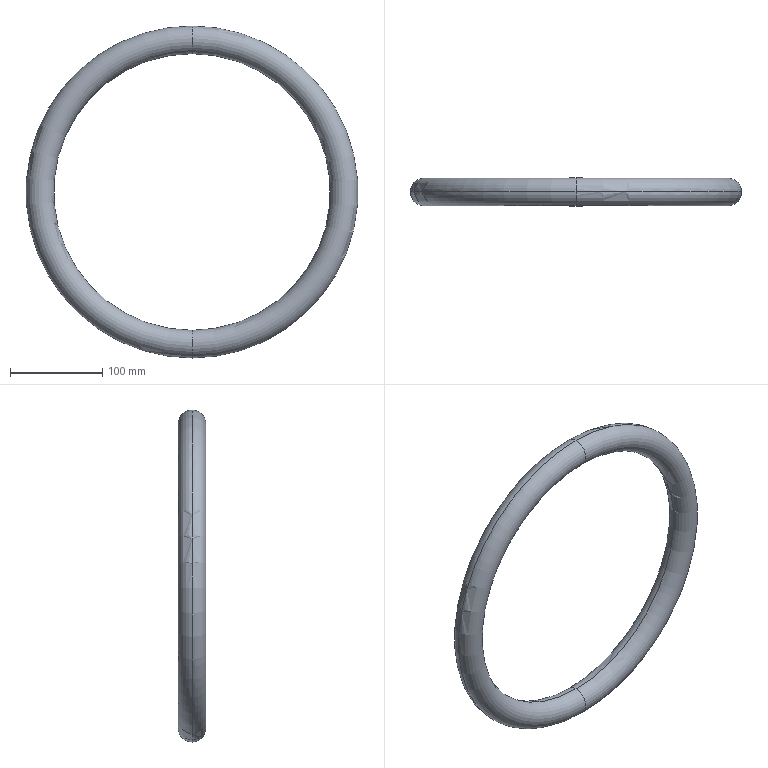Part | SolidWorks | features RefAxis 1, Revolution 1 | 1 solid | 4 faces | box 360 x 30 x 360 mm | volume 732818 mm3 | torus 4
STEP:
#1=CARTESIAN_POINT('',(0.,0.,180.));
#2=VERTEX_POINT('',#1);
#3=CARTESIAN_POINT('',(0.,0.,150.));
#4=VERTEX_POINT('',#3);
#5=CARTESIAN_POINT('',(0.,0.,165.));
#6=DIRECTION('',(1.,0.,0.));
#7=DIRECTION('',(0.,0.,-1.));
#8=AXIS2_PLACEMENT_3D('',#5,#6,#7);
#9=CIRCLE('',#8,15.);
#10=EDGE_CURVE('',#2,#4,#9,.T.);
#11=ORIENTED_EDGE('',*,*,#10,.F.);
#12=CARTESIAN_POINT('',(0.,0.,-180.));
#13=VERTEX_POINT('',#12);
#14=CARTESIAN_POINT('',(0.,0.,0.));
#15=DIRECTION('',(0.,-1.,0.));
#16=DIRECTION('',(0.,0.,-1.));
#17=AXIS2_PLACEMENT_3D('',#14,#15,#16);
#18=CIRCLE('',#17,180.);
#19=EDGE_CURVE('',#2,#13,#18,.T.);
#20=ORIENTED_EDGE('',*,*,#19,.T.);
#21=CARTESIAN_POINT('',(0.,0.,-150.));
#22=VERTEX_POINT('',#21);
#23=CARTESIAN_POINT('',(0.,0.,-165.));
#24=DIRECTION('',(-1.,0.,0.));
#25=DIRECTION('',(0.,0.,1.));
#26=AXIS2_PLACEMENT_3D('',#23,#24,#25);
#27=CIRCLE('',#26,15.);
#28=EDGE_CURVE('',#13,#22,#27,.T.);
#29=ORIENTED_EDGE('',*,*,#28,.T.);
#30=CARTESIAN_POINT('',(0.,0.,0.));
#31=DIRECTION('',(0.,-1.,0.));
#32=DIRECTION('',(0.,0.,-1.));
#33=AXIS2_PLACEMENT_3D('',#30,#31,#32);
#34=CIRCLE('',#33,150.);
#35=EDGE_CURVE('',#4,#22,#34,.T.);
#36=ORIENTED_EDGE('',*,*,#35,.F.);
#37=EDGE_LOOP('',(#11,#20,#29,#36));
#38=FACE_OUTER_BOUND('',#37,.T.);
#39=CARTESIAN_POINT('',(0.,0.,0.));
#40=DIRECTION('',(0.,-1.,0.));
#41=DIRECTION('',(0.,0.,-1.));
#42=AXIS2_PLACEMENT_3D('',#39,#40,#41);
#43=TOROIDAL_SURFACE('',#42,165.,15.);
#44=ADVANCED_FACE('',(#38),#43,.T.);
#45=ORIENTED_EDGE('',*,*,#28,.F.);
#46=CARTESIAN_POINT('',(0.,0.,0.));
#47=DIRECTION('',(0.,-1.,0.));
#48=DIRECTION('',(0.,0.,-1.));
#49=AXIS2_PLACEMENT_3D('',#46,#47,#48);
#50=CIRCLE('',#49,180.);
#51=EDGE_CURVE('',#13,#2,#50,.T.);
#52=ORIENTED_EDGE('',*,*,#51,.T.);
#53=ORIENTED_EDGE('',*,*,#10,.T.);
#54=CARTESIAN_POINT('',(0.,0.,0.));
#55=DIRECTION('',(0.,-1.,0.));
#56=DIRECTION('',(0.,0.,-1.));
#57=AXIS2_PLACEMENT_3D('',#54,#55,#56);
#58=CIRCLE('',#57,150.);
#59=EDGE_CURVE('',#22,#4,#58,.T.);
#60=ORIENTED_EDGE('',*,*,#59,.F.);
#61=EDGE_LOOP('',(#45,#52,#53,#60));
#62=FACE_OUTER_BOUND('',#61,.T.);
#63=CARTESIAN_POINT('',(0.,0.,0.));
#64=DIRECTION('',(0.,-1.,0.));
#65=DIRECTION('',(0.,0.,-1.));
#66=AXIS2_PLACEMENT_3D('',#63,#64,#65);
#67=TOROIDAL_SURFACE('',#66,165.,15.);
#68=ADVANCED_FACE('',(#62),#67,.T.);
#69=ORIENTED_EDGE('',*,*,#51,.F.);
#70=CARTESIAN_POINT('',(0.,0.,-165.));
#71=DIRECTION('',(-1.,0.,0.));
#72=DIRECTION('',(0.,0.,1.));
#73=AXIS2_PLACEMENT_3D('',#70,#71,#72);
#74=CIRCLE('',#73,15.);
#75=EDGE_CURVE('',#22,#13,#74,.T.);
#76=ORIENTED_EDGE('',*,*,#75,.F.);
#77=ORIENTED_EDGE('',*,*,#59,.T.);
#78=CARTESIAN_POINT('',(0.,0.,165.));
#79=DIRECTION('',(1.,0.,0.));
#80=DIRECTION('',(0.,0.,-1.));
#81=AXIS2_PLACEMENT_3D('',#78,#79,#80);
#82=CIRCLE('',#81,15.);
#83=EDGE_CURVE('',#4,#2,#82,.T.);
#84=ORIENTED_EDGE('',*,*,#83,.T.);
#85=EDGE_LOOP('',(#69,#76,#77,#84));
#86=FACE_OUTER_BOUND('',#85,.T.);
#87=CARTESIAN_POINT('',(0.,0.,0.));
#88=DIRECTION('',(0.,-1.,0.));
#89=DIRECTION('',(0.,0.,-1.));
#90=AXIS2_PLACEMENT_3D('',#87,#88,#89);
#91=TOROIDAL_SURFACE('',#90,165.,15.);
#92=ADVANCED_FACE('',(#86),#91,.T.);
#93=ORIENTED_EDGE('',*,*,#19,.F.);
#94=ORIENTED_EDGE('',*,*,#83,.F.);
#95=ORIENTED_EDGE('',*,*,#35,.T.);
#96=ORIENTED_EDGE('',*,*,#75,.T.);
#97=EDGE_LOOP('',(#93,#94,#95,#96));
#98=FACE_OUTER_BOUND('',#97,.T.);
#99=CARTESIAN_POINT('',(0.,0.,0.));
#100=DIRECTION('',(0.,-1.,0.));
#101=DIRECTION('',(0.,0.,-1.));
#102=AXIS2_PLACEMENT_3D('',#99,#100,#101);
#103=TOROIDAL_SURFACE('',#102,165.,15.);
#104=ADVANCED_FACE('',(#98),#103,.T.);
#105=CLOSED_SHELL('',(#44,#68,#92,#104));
#106=MANIFOLD_SOLID_BREP('',#105);
#107=CARTESIAN_POINT('',(0.,0.,0.));
#108=DIRECTION('',(0.,0.,1.));
#109=DIRECTION('',(1.,0.,0.));
#110=AXIS2_PLACEMENT_3D('',#107,#108,#109);
#111=(LENGTH_UNIT()NAMED_UNIT(*)SI_UNIT(.MILLI.,.METRE.));
#112=UNCERTAINTY_MEASURE_WITH_UNIT(LENGTH_MEASURE(0.00001),#111,'','');
#113=(NAMED_UNIT(*)PLANE_ANGLE_UNIT()SI_UNIT($,.RADIAN.));
#114=(NAMED_UNIT(*)SI_UNIT($,.STERADIAN.)SOLID_ANGLE_UNIT());
#115=(GEOMETRIC_REPRESENTATION_CONTEXT(3)GLOBAL_UNCERTAINTY_ASSIGNED_CONTEXT((#112))GLOBAL_UNIT_ASSIGNED_CONTEXT((#111,#113,#114))REPRESENTATION_CONTEXT('',''));
#116=ADVANCED_BREP_SHAPE_REPRESENTATION('',(#106,#110),#115);